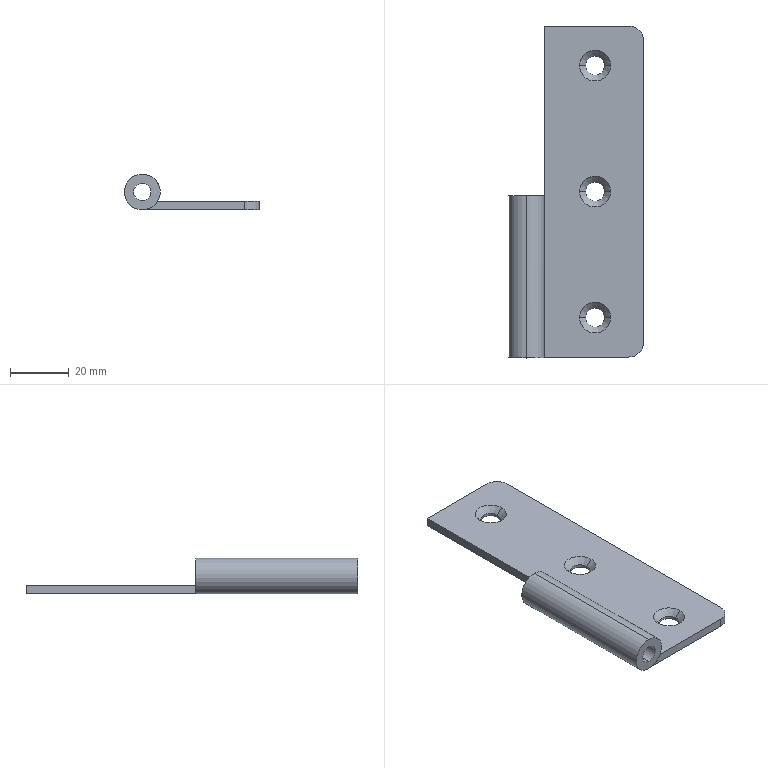Part | SolidWorks | features BaseBody 1 | 1 solid | 26 faces | box 46.1 x 113.3 x 12.2 mm | volume 16282 mm3 | cylinder 12 | plane 8 | cone 6 | commonest cylinder face diameters 6.5 x6 6 x2 10 x2 12.2 x2
STEP:
#1=CARTESIAN_POINT('',(20.25,43.,-6.1));
#2=VERTEX_POINT('',#1);
#3=CARTESIAN_POINT('',(26.75,43.,-6.1));
#4=VERTEX_POINT('',#3);
#5=CARTESIAN_POINT('',(23.5,43.,-6.1));
#6=DIRECTION('',(0.,0.,1.));
#7=DIRECTION('',(1.,0.,0.));
#8=AXIS2_PLACEMENT_3D('',#5,#6,#7);
#9=CIRCLE('',#8,3.25);
#10=EDGE_CURVE('',#2,#4,#9,.T.);
#11=ORIENTED_EDGE('',*,*,#10,.F.);
#12=CARTESIAN_POINT('',(20.25,43.,-5.15));
#13=VERTEX_POINT('',#12);
#14=CARTESIAN_POINT('',(20.25,43.,-3.1));
#15=DIRECTION('',(0.,0.,1.));
#16=VECTOR('',#15,1000.);
#17=LINE('',#14,#16);
#18=EDGE_CURVE('',#2,#13,#17,.T.);
#19=ORIENTED_EDGE('',*,*,#18,.T.);
#20=CARTESIAN_POINT('',(26.75,43.,-5.15));
#21=VERTEX_POINT('',#20);
#22=CARTESIAN_POINT('',(23.5,43.,-5.15));
#23=DIRECTION('',(0.,0.,1.));
#24=DIRECTION('',(1.,0.,0.));
#25=AXIS2_PLACEMENT_3D('',#22,#23,#24);
#26=CIRCLE('',#25,3.25);
#27=EDGE_CURVE('',#13,#21,#26,.T.);
#28=ORIENTED_EDGE('',*,*,#27,.T.);
#29=CARTESIAN_POINT('',(26.75,43.,-3.1));
#30=DIRECTION('',(0.,0.,1.));
#31=VECTOR('',#30,1000.);
#32=LINE('',#29,#31);
#33=EDGE_CURVE('',#4,#21,#32,.T.);
#34=ORIENTED_EDGE('',*,*,#33,.F.);
#35=EDGE_LOOP('',(#11,#19,#28,#34));
#36=FACE_OUTER_BOUND('',#35,.T.);
#37=CARTESIAN_POINT('',(23.5,43.,-3.1));
#38=DIRECTION('',(0.,0.,1.));
#39=DIRECTION('',(1.,0.,0.));
#40=AXIS2_PLACEMENT_3D('',#37,#38,#39);
#41=CYLINDRICAL_SURFACE('',#40,3.25);
#42=ADVANCED_FACE('',(#36),#41,.F.);
#43=CARTESIAN_POINT('',(20.25,0.,-6.1));
#44=VERTEX_POINT('',#43);
#45=CARTESIAN_POINT('',(26.75,0.,-6.1));
#46=VERTEX_POINT('',#45);
#47=CARTESIAN_POINT('',(23.5,0.,-6.1));
#48=DIRECTION('',(0.,0.,1.));
#49=DIRECTION('',(1.,0.,0.));
#50=AXIS2_PLACEMENT_3D('',#47,#48,#49);
#51=CIRCLE('',#50,3.25);
#52=EDGE_CURVE('',#44,#46,#51,.T.);
#53=ORIENTED_EDGE('',*,*,#52,.F.);
#54=CARTESIAN_POINT('',(20.25,0.,-5.15));
#55=VERTEX_POINT('',#54);
#56=CARTESIAN_POINT('',(20.25,0.,-3.1));
#57=DIRECTION('',(0.,0.,1.));
#58=VECTOR('',#57,1000.);
#59=LINE('',#56,#58);
#60=EDGE_CURVE('',#44,#55,#59,.T.);
#61=ORIENTED_EDGE('',*,*,#60,.T.);
#62=CARTESIAN_POINT('',(26.75,0.,-5.15));
#63=VERTEX_POINT('',#62);
#64=CARTESIAN_POINT('',(23.5,0.,-5.15));
#65=DIRECTION('',(0.,0.,1.));
#66=DIRECTION('',(1.,0.,0.));
#67=AXIS2_PLACEMENT_3D('',#64,#65,#66);
#68=CIRCLE('',#67,3.25);
#69=EDGE_CURVE('',#55,#63,#68,.T.);
#70=ORIENTED_EDGE('',*,*,#69,.T.);
#71=CARTESIAN_POINT('',(26.75,0.,-3.1));
#72=DIRECTION('',(0.,0.,1.));
#73=VECTOR('',#72,1000.);
#74=LINE('',#71,#73);
#75=EDGE_CURVE('',#46,#63,#74,.T.);
#76=ORIENTED_EDGE('',*,*,#75,.F.);
#77=EDGE_LOOP('',(#53,#61,#70,#76));
#78=FACE_OUTER_BOUND('',#77,.T.);
#79=CARTESIAN_POINT('',(23.5,0.,-3.1));
#80=DIRECTION('',(0.,0.,1.));
#81=DIRECTION('',(1.,0.,0.));
#82=AXIS2_PLACEMENT_3D('',#79,#80,#81);
#83=CYLINDRICAL_SURFACE('',#82,3.25);
#84=ADVANCED_FACE('',(#78),#83,.F.);
#85=CARTESIAN_POINT('',(20.25,-43.,-6.1));
#86=VERTEX_POINT('',#85);
#87=CARTESIAN_POINT('',(26.75,-43.,-6.1));
#88=VERTEX_POINT('',#87);
#89=CARTESIAN_POINT('',(23.5,-43.,-6.1));
#90=DIRECTION('',(0.,0.,1.));
#91=DIRECTION('',(1.,0.,0.));
#92=AXIS2_PLACEMENT_3D('',#89,#90,#91);
#93=CIRCLE('',#92,3.25);
#94=EDGE_CURVE('',#86,#88,#93,.T.);
#95=ORIENTED_EDGE('',*,*,#94,.F.);
#96=CARTESIAN_POINT('',(20.25,-43.,-5.15));
#97=VERTEX_POINT('',#96);
#98=CARTESIAN_POINT('',(20.25,-43.,-3.1));
#99=DIRECTION('',(0.,0.,1.));
#100=VECTOR('',#99,1000.);
#101=LINE('',#98,#100);
#102=EDGE_CURVE('',#86,#97,#101,.T.);
#103=ORIENTED_EDGE('',*,*,#102,.T.);
#104=CARTESIAN_POINT('',(26.75,-43.,-5.15));
#105=VERTEX_POINT('',#104);
#106=CARTESIAN_POINT('',(23.5,-43.,-5.15));
#107=DIRECTION('',(0.,0.,1.));
#108=DIRECTION('',(1.,0.,0.));
#109=AXIS2_PLACEMENT_3D('',#106,#107,#108);
#110=CIRCLE('',#109,3.25);
#111=EDGE_CURVE('',#97,#105,#110,.T.);
#112=ORIENTED_EDGE('',*,*,#111,.T.);
#113=CARTESIAN_POINT('',(26.75,-43.,-3.1));
#114=DIRECTION('',(0.,0.,1.));
#115=VECTOR('',#114,1000.);
#116=LINE('',#113,#115);
#117=EDGE_CURVE('',#88,#105,#116,.T.);
#118=ORIENTED_EDGE('',*,*,#117,.F.);
#119=EDGE_LOOP('',(#95,#103,#112,#118));
#120=FACE_OUTER_BOUND('',#119,.T.);
#121=CARTESIAN_POINT('',(23.5,-43.,-3.1));
#122=DIRECTION('',(0.,0.,1.));
#123=DIRECTION('',(1.,0.,0.));
#124=AXIS2_PLACEMENT_3D('',#121,#122,#123);
#125=CYLINDRICAL_SURFACE('',#124,3.25);
#126=ADVANCED_FACE('',(#120),#125,.F.);
#127=ORIENTED_EDGE('',*,*,#27,.F.);
#128=CARTESIAN_POINT('',(18.2,43.,-3.1));
#129=VERTEX_POINT('',#128);
#130=CARTESIAN_POINT('',(20.25,43.,-5.15));
#131=DIRECTION('',(-0.7071,0.,0.7071));
#132=VECTOR('',#131,1000.);
#133=LINE('',#130,#132);
#134=EDGE_CURVE('',#13,#129,#133,.T.);
#135=ORIENTED_EDGE('',*,*,#134,.T.);
#136=CARTESIAN_POINT('',(28.8,43.,-3.1));
#137=VERTEX_POINT('',#136);
#138=CARTESIAN_POINT('',(23.5,43.,-3.1));
#139=DIRECTION('',(0.,0.,1.));
#140=DIRECTION('',(1.,0.,0.));
#141=AXIS2_PLACEMENT_3D('',#138,#139,#140);
#142=CIRCLE('',#141,5.3);
#143=EDGE_CURVE('',#129,#137,#142,.T.);
#144=ORIENTED_EDGE('',*,*,#143,.T.);
#145=CARTESIAN_POINT('',(26.75,43.,-5.15));
#146=DIRECTION('',(0.7071,0.,0.7071));
#147=VECTOR('',#146,1000.);
#148=LINE('',#145,#147);
#149=EDGE_CURVE('',#21,#137,#148,.T.);
#150=ORIENTED_EDGE('',*,*,#149,.F.);
#151=EDGE_LOOP('',(#127,#135,#144,#150));
#152=FACE_OUTER_BOUND('',#151,.T.);
#153=CARTESIAN_POINT('',(23.5,43.,-5.15));
#154=DIRECTION('',(0.,0.,1.));
#155=DIRECTION('',(1.,0.,0.));
#156=AXIS2_PLACEMENT_3D('',#153,#154,#155);
#157=CONICAL_SURFACE('',#156,3.25,0.7854);
#158=ADVANCED_FACE('',(#152),#157,.F.);
#159=ORIENTED_EDGE('',*,*,#69,.F.);
#160=CARTESIAN_POINT('',(18.2,0.,-3.1));
#161=VERTEX_POINT('',#160);
#162=CARTESIAN_POINT('',(20.25,0.,-5.15));
#163=DIRECTION('',(-0.7071,0.,0.7071));
#164=VECTOR('',#163,1000.);
#165=LINE('',#162,#164);
#166=EDGE_CURVE('',#55,#161,#165,.T.);
#167=ORIENTED_EDGE('',*,*,#166,.T.);
#168=CARTESIAN_POINT('',(28.8,0.,-3.1));
#169=VERTEX_POINT('',#168);
#170=CARTESIAN_POINT('',(23.5,0.,-3.1));
#171=DIRECTION('',(0.,0.,1.));
#172=DIRECTION('',(1.,0.,0.));
#173=AXIS2_PLACEMENT_3D('',#170,#171,#172);
#174=CIRCLE('',#173,5.3);
#175=EDGE_CURVE('',#161,#169,#174,.T.);
#176=ORIENTED_EDGE('',*,*,#175,.T.);
#177=CARTESIAN_POINT('',(26.75,0.,-5.15));
#178=DIRECTION('',(0.7071,0.,0.7071));
#179=VECTOR('',#178,1000.);
#180=LINE('',#177,#179);
#181=EDGE_CURVE('',#63,#169,#180,.T.);
#182=ORIENTED_EDGE('',*,*,#181,.F.);
#183=EDGE_LOOP('',(#159,#167,#176,#182));
#184=FACE_OUTER_BOUND('',#183,.T.);
#185=CARTESIAN_POINT('',(23.5,0.,-5.15));
#186=DIRECTION('',(0.,0.,1.));
#187=DIRECTION('',(1.,0.,0.));
#188=AXIS2_PLACEMENT_3D('',#185,#186,#187);
#189=CONICAL_SURFACE('',#188,3.25,0.7854);
#190=ADVANCED_FACE('',(#184),#189,.F.);
#191=ORIENTED_EDGE('',*,*,#111,.F.);
#192=CARTESIAN_POINT('',(18.2,-43.,-3.1));
#193=VERTEX_POINT('',#192);
#194=CARTESIAN_POINT('',(20.25,-43.,-5.15));
#195=DIRECTION('',(-0.7071,0.,0.7071));
#196=VECTOR('',#195,1000.);
#197=LINE('',#194,#196);
#198=EDGE_CURVE('',#97,#193,#197,.T.);
#199=ORIENTED_EDGE('',*,*,#198,.T.);
#200=CARTESIAN_POINT('',(28.8,-43.,-3.1));
#201=VERTEX_POINT('',#200);
#202=CARTESIAN_POINT('',(23.5,-43.,-3.1));
#203=DIRECTION('',(0.,0.,1.));
#204=DIRECTION('',(1.,0.,0.));
#205=AXIS2_PLACEMENT_3D('',#202,#203,#204);
#206=CIRCLE('',#205,5.3);
#207=EDGE_CURVE('',#193,#201,#206,.T.);
#208=ORIENTED_EDGE('',*,*,#207,.T.);
#209=CARTESIAN_POINT('',(26.75,-43.,-5.15));
#210=DIRECTION('',(0.7071,0.,0.7071));
#211=VECTOR('',#210,1000.);
#212=LINE('',#209,#211);
#213=EDGE_CURVE('',#105,#201,#212,.T.);
#214=ORIENTED_EDGE('',*,*,#213,.F.);
#215=EDGE_LOOP('',(#191,#199,#208,#214));
#216=FACE_OUTER_BOUND('',#215,.T.);
#217=CARTESIAN_POINT('',(23.5,-43.,-5.15));
#218=DIRECTION('',(0.,0.,1.));
#219=DIRECTION('',(1.,0.,0.));
#220=AXIS2_PLACEMENT_3D('',#217,#218,#219);
#221=CONICAL_SURFACE('',#220,3.25,0.7854);
#222=ADVANCED_FACE('',(#216),#221,.F.);
#223=CARTESIAN_POINT('',(0.,-1.5,3.));
#224=VERTEX_POINT('',#223);
#225=CARTESIAN_POINT('',(0.,-1.5,-3.));
#226=VERTEX_POINT('',#225);
#227=CARTESIAN_POINT('',(0.,-1.5,0.));
#228=DIRECTION('',(0.,-1.,0.));
#229=DIRECTION('',(0.,0.,1.));
#230=AXIS2_PLACEMENT_3D('',#227,#228,#229);
#231=CIRCLE('',#230,3.);
#232=EDGE_CURVE('',#224,#226,#231,.T.);
#233=ORIENTED_EDGE('',*,*,#232,.F.);
#234=CARTESIAN_POINT('',(0.,-56.8,3.));
#235=VERTEX_POINT('',#234);
#236=CARTESIAN_POINT('',(0.,-56.8,3.));
#237=DIRECTION('',(0.,-1.,0.));
#238=VECTOR('',#237,1000.);
#239=LINE('',#236,#238);
#240=EDGE_CURVE('',#224,#235,#239,.T.);
#241=ORIENTED_EDGE('',*,*,#240,.T.);
#242=CARTESIAN_POINT('',(0.,-56.8,-3.));
#243=VERTEX_POINT('',#242);
#244=CARTESIAN_POINT('',(0.,-56.8,0.));
#245=DIRECTION('',(0.,-1.,0.));
#246=DIRECTION('',(0.,0.,-1.));
#247=AXIS2_PLACEMENT_3D('',#244,#245,#246);
#248=CIRCLE('',#247,3.);
#249=EDGE_CURVE('',#235,#243,#248,.T.);
#250=ORIENTED_EDGE('',*,*,#249,.T.);
#251=CARTESIAN_POINT('',(0.,-56.8,-3.));
#252=DIRECTION('',(0.,-1.,0.));
#253=VECTOR('',#252,1000.);
#254=LINE('',#251,#253);
#255=EDGE_CURVE('',#226,#243,#254,.T.);
#256=ORIENTED_EDGE('',*,*,#255,.F.);
#257=EDGE_LOOP('',(#233,#241,#250,#256));
#258=FACE_OUTER_BOUND('',#257,.T.);
#259=CARTESIAN_POINT('',(0.,-56.8,0.));
#260=DIRECTION('',(0.,-1.,0.));
#261=DIRECTION('',(0.,0.,-1.));
#262=AXIS2_PLACEMENT_3D('',#259,#260,#261);
#263=CYLINDRICAL_SURFACE('',#262,3.);
#264=ADVANCED_FACE('',(#258),#263,.F.);
#265=CARTESIAN_POINT('',(0.,-1.5,6.1));
#266=VERTEX_POINT('',#265);
#267=CARTESIAN_POINT('',(5.254,-1.5,-3.1));
#268=VERTEX_POINT('',#267);
#269=CARTESIAN_POINT('',(0.,-1.5,0.));
#270=DIRECTION('',(0.,1.,0.));
#271=DIRECTION('',(0.,0.,-1.));
#272=AXIS2_PLACEMENT_3D('',#269,#270,#271);
#273=CIRCLE('',#272,6.1);
#274=EDGE_CURVE('',#266,#268,#273,.T.);
#275=ORIENTED_EDGE('',*,*,#274,.F.);
#276=CARTESIAN_POINT('',(0.,-56.8,6.1));
#277=VERTEX_POINT('',#276);
#278=CARTESIAN_POINT('',(0.,-56.8,6.1));
#279=DIRECTION('',(0.,-1.,0.));
#280=VECTOR('',#279,1000.);
#281=LINE('',#278,#280);
#282=EDGE_CURVE('',#266,#277,#281,.T.);
#283=ORIENTED_EDGE('',*,*,#282,.T.);
#284=CARTESIAN_POINT('',(0.,-56.8,-6.1));
#285=VERTEX_POINT('',#284);
#286=CARTESIAN_POINT('',(0.,-56.8,0.));
#287=DIRECTION('',(0.,-1.,0.));
#288=DIRECTION('',(0.,0.,-1.));
#289=AXIS2_PLACEMENT_3D('',#286,#287,#288);
#290=CIRCLE('',#289,6.1);
#291=EDGE_CURVE('',#285,#277,#290,.T.);
#292=ORIENTED_EDGE('',*,*,#291,.F.);
#293=CARTESIAN_POINT('',(0.,-56.5,-6.1));
#294=VERTEX_POINT('',#293);
#295=CARTESIAN_POINT('',(0.,-56.8,-6.1));
#296=DIRECTION('',(0.,-1.,0.));
#297=VECTOR('',#296,1000.);
#298=LINE('',#295,#297);
#299=EDGE_CURVE('',#294,#285,#298,.T.);
#300=ORIENTED_EDGE('',*,*,#299,.F.);
#301=CARTESIAN_POINT('',(5.254,-56.5,-3.1));
#302=VERTEX_POINT('',#301);
#303=CARTESIAN_POINT('',(0.,-56.5,0.));
#304=DIRECTION('',(0.,1.,0.));
#305=DIRECTION('',(0.8612,0.,-0.5082));
#306=AXIS2_PLACEMENT_3D('',#303,#304,#305);
#307=CIRCLE('',#306,6.1);
#308=EDGE_CURVE('',#302,#294,#307,.T.);
#309=ORIENTED_EDGE('',*,*,#308,.F.);
#310=CARTESIAN_POINT('',(5.254,-56.5,-3.1));
#311=DIRECTION('',(0.,1.,0.));
#312=VECTOR('',#311,1000.);
#313=LINE('',#310,#312);
#314=EDGE_CURVE('',#302,#268,#313,.T.);
#315=ORIENTED_EDGE('',*,*,#314,.T.);
#316=EDGE_LOOP('',(#275,#283,#292,#300,#309,#315));
#317=FACE_OUTER_BOUND('',#316,.T.);
#318=CARTESIAN_POINT('',(0.,-56.8,0.));
#319=DIRECTION('',(0.,-1.,0.));
#320=DIRECTION('',(0.,0.,-1.));
#321=AXIS2_PLACEMENT_3D('',#318,#319,#320);
#322=CYLINDRICAL_SURFACE('',#321,6.1);
#323=ADVANCED_FACE('',(#317),#322,.T.);
#324=ORIENTED_EDGE('',*,*,#282,.F.);
#325=CARTESIAN_POINT('',(0.,-1.5,-6.1));
#326=VERTEX_POINT('',#325);
#327=CARTESIAN_POINT('',(0.,-1.5,0.));
#328=DIRECTION('',(0.,1.,0.));
#329=DIRECTION('',(0.,0.,-1.));
#330=AXIS2_PLACEMENT_3D('',#327,#328,#329);
#331=CIRCLE('',#330,6.1);
#332=EDGE_CURVE('',#326,#266,#331,.T.);
#333=ORIENTED_EDGE('',*,*,#332,.F.);
#334=CARTESIAN_POINT('',(0.,-1.5,-6.1));
#335=DIRECTION('',(0.,-1.,0.));
#336=VECTOR('',#335,1000.);
#337=LINE('',#334,#336);
#338=EDGE_CURVE('',#326,#294,#337,.T.);
#339=ORIENTED_EDGE('',*,*,#338,.T.);
#340=ORIENTED_EDGE('',*,*,#299,.T.);
#341=CARTESIAN_POINT('',(0.,-56.8,0.));
#342=DIRECTION('',(0.,-1.,0.));
#343=DIRECTION('',(0.,0.,-1.));
#344=AXIS2_PLACEMENT_3D('',#341,#342,#343);
#345=CIRCLE('',#344,6.1);
#346=EDGE_CURVE('',#277,#285,#345,.T.);
#347=ORIENTED_EDGE('',*,*,#346,.F.);
#348=EDGE_LOOP('',(#324,#333,#339,#340,#347));
#349=FACE_OUTER_BOUND('',#348,.T.);
#350=CARTESIAN_POINT('',(0.,-56.8,0.));
#351=DIRECTION('',(0.,-1.,0.));
#352=DIRECTION('',(0.,0.,-1.));
#353=AXIS2_PLACEMENT_3D('',#350,#351,#352);
#354=CYLINDRICAL_SURFACE('',#353,6.1);
#355=ADVANCED_FACE('',(#349),#354,.T.);
#356=CARTESIAN_POINT('',(0.,-56.8,0.));
#357=DIRECTION('',(0.,-1.,0.));
#358=DIRECTION('',(0.,0.,-1.));
#359=AXIS2_PLACEMENT_3D('',#356,#357,#358);
#360=CIRCLE('',#359,3.);
#361=EDGE_CURVE('',#243,#235,#360,.T.);
#362=ORIENTED_EDGE('',*,*,#361,.F.);
#363=ORIENTED_EDGE('',*,*,#249,.F.);
#364=EDGE_LOOP('',(#362,#363));
#365=FACE_BOUND('',#364,.T.);
#366=ORIENTED_EDGE('',*,*,#291,.T.);
#367=ORIENTED_EDGE('',*,*,#346,.T.);
#368=EDGE_LOOP('',(#366,#367));
#369=FACE_OUTER_BOUND('',#368,.T.);
#370=CARTESIAN_POINT('',(6.1,-56.8,0.));
#371=DIRECTION('',(0.,1.,0.));
#372=DIRECTION('',(0.,0.,1.));
#373=AXIS2_PLACEMENT_3D('',#370,#371,#372);
#374=PLANE('',#373);
#375=ADVANCED_FACE('',(#365,#369),#374,.F.);
#376=CARTESIAN_POINT('',(23.5,-43.,-3.1));
#377=DIRECTION('',(0.,0.,1.));
#378=DIRECTION('',(1.,0.,0.));
#379=AXIS2_PLACEMENT_3D('',#376,#377,#378);
#380=CIRCLE('',#379,5.3);
#381=EDGE_CURVE('',#201,#193,#380,.T.);
#382=ORIENTED_EDGE('',*,*,#381,.F.);
#383=ORIENTED_EDGE('',*,*,#207,.F.);
#384=EDGE_LOOP('',(#382,#383));
#385=FACE_BOUND('',#384,.T.);
#386=CARTESIAN_POINT('',(23.5,0.,-3.1));
#387=DIRECTION('',(0.,0.,1.));
#388=DIRECTION('',(1.,0.,0.));
#389=AXIS2_PLACEMENT_3D('',#386,#387,#388);
#390=CIRCLE('',#389,5.3);
#391=EDGE_CURVE('',#169,#161,#390,.T.);
#392=ORIENTED_EDGE('',*,*,#391,.F.);
#393=ORIENTED_EDGE('',*,*,#175,.F.);
#394=EDGE_LOOP('',(#392,#393));
#395=FACE_BOUND('',#394,.T.);
#396=CARTESIAN_POINT('',(23.5,43.,-3.1));
#397=DIRECTION('',(0.,0.,1.));
#398=DIRECTION('',(1.,0.,0.));
#399=AXIS2_PLACEMENT_3D('',#396,#397,#398);
#400=CIRCLE('',#399,5.3);
#401=EDGE_CURVE('',#137,#129,#400,.T.);
#402=ORIENTED_EDGE('',*,*,#401,.F.);
#403=ORIENTED_EDGE('',*,*,#143,.F.);
#404=EDGE_LOOP('',(#402,#403));
#405=FACE_BOUND('',#404,.T.);
#406=CARTESIAN_POINT('',(6.2,56.5,-3.1));
#407=VERTEX_POINT('',#406);
#408=CARTESIAN_POINT('',(6.2,-1.5,-3.1));
#409=VERTEX_POINT('',#408);
#410=CARTESIAN_POINT('',(6.2,56.5,-3.1));
#411=DIRECTION('',(0.,-1.,0.));
#412=VECTOR('',#411,1000.);
#413=LINE('',#410,#412);
#414=EDGE_CURVE('',#407,#409,#413,.T.);
#415=ORIENTED_EDGE('',*,*,#414,.T.);
#416=CARTESIAN_POINT('',(6.2,-1.5,-3.1));
#417=DIRECTION('',(-1.,0.,0.));
#418=VECTOR('',#417,1000.);
#419=LINE('',#416,#418);
#420=EDGE_CURVE('',#409,#268,#419,.T.);
#421=ORIENTED_EDGE('',*,*,#420,.T.);
#422=ORIENTED_EDGE('',*,*,#314,.F.);
#423=CARTESIAN_POINT('',(35.,-56.5,-3.1));
#424=VERTEX_POINT('',#423);
#425=CARTESIAN_POINT('',(5.254,-56.5,-3.1));
#426=DIRECTION('',(1.,0.,0.));
#427=VECTOR('',#426,1000.);
#428=LINE('',#425,#427);
#429=EDGE_CURVE('',#302,#424,#428,.T.);
#430=ORIENTED_EDGE('',*,*,#429,.T.);
#431=CARTESIAN_POINT('',(40.,-51.5,-3.1));
#432=VERTEX_POINT('',#431);
#433=CARTESIAN_POINT('',(35.,-51.5,-3.1));
#434=DIRECTION('',(0.,0.,1.));
#435=DIRECTION('',(0.,-1.,0.));
#436=AXIS2_PLACEMENT_3D('',#433,#434,#435);
#437=CIRCLE('',#436,5.);
#438=EDGE_CURVE('',#424,#432,#437,.T.);
#439=ORIENTED_EDGE('',*,*,#438,.T.);
#440=CARTESIAN_POINT('',(40.,51.5,-3.1));
#441=VERTEX_POINT('',#440);
#442=CARTESIAN_POINT('',(40.,-51.5,-3.1));
#443=DIRECTION('',(0.,1.,0.));
#444=VECTOR('',#443,1000.);
#445=LINE('',#442,#444);
#446=EDGE_CURVE('',#432,#441,#445,.T.);
#447=ORIENTED_EDGE('',*,*,#446,.T.);
#448=CARTESIAN_POINT('',(35.,56.5,-3.1));
#449=VERTEX_POINT('',#448);
#450=CARTESIAN_POINT('',(35.,51.5,-3.1));
#451=DIRECTION('',(0.,0.,1.));
#452=DIRECTION('',(1.,0.,0.));
#453=AXIS2_PLACEMENT_3D('',#450,#451,#452);
#454=CIRCLE('',#453,5.);
#455=EDGE_CURVE('',#441,#449,#454,.T.);
#456=ORIENTED_EDGE('',*,*,#455,.T.);
#457=CARTESIAN_POINT('',(35.,56.5,-3.1));
#458=DIRECTION('',(-1.,0.,0.));
#459=VECTOR('',#458,1000.);
#460=LINE('',#457,#459);
#461=EDGE_CURVE('',#449,#407,#460,.T.);
#462=ORIENTED_EDGE('',*,*,#461,.T.);
#463=EDGE_LOOP('',(#415,#421,#422,#430,#439,#447,#456,#462));
#464=FACE_OUTER_BOUND('',#463,.T.);
#465=CARTESIAN_POINT('',(35.,-51.5,-3.1));
#466=DIRECTION('',(0.,0.,1.));
#467=DIRECTION('',(1.,0.,0.));
#468=AXIS2_PLACEMENT_3D('',#465,#466,#467);
#469=PLANE('',#468);
#470=ADVANCED_FACE('',(#385,#395,#405,#464),#469,.T.);
#471=CARTESIAN_POINT('',(0.,-1.5,0.));
#472=DIRECTION('',(0.,-1.,0.));
#473=DIRECTION('',(0.,0.,1.));
#474=AXIS2_PLACEMENT_3D('',#471,#472,#473);
#475=CIRCLE('',#474,3.);
#476=EDGE_CURVE('',#226,#224,#475,.T.);
#477=ORIENTED_EDGE('',*,*,#476,.T.);
#478=ORIENTED_EDGE('',*,*,#232,.T.);
#479=EDGE_LOOP('',(#477,#478));
#480=FACE_BOUND('',#479,.T.);
#481=CARTESIAN_POINT('',(6.2,-1.5,-6.1));
#482=VERTEX_POINT('',#481);
#483=CARTESIAN_POINT('',(6.2,-1.5,-3.1));
#484=DIRECTION('',(0.,0.,-1.));
#485=VECTOR('',#484,1000.);
#486=LINE('',#483,#485);
#487=EDGE_CURVE('',#409,#482,#486,.T.);
#488=ORIENTED_EDGE('',*,*,#487,.T.);
#489=CARTESIAN_POINT('',(6.2,-1.5,-6.1));
#490=DIRECTION('',(-1.,0.,0.));
#491=VECTOR('',#490,1000.);
#492=LINE('',#489,#491);
#493=EDGE_CURVE('',#482,#326,#492,.T.);
#494=ORIENTED_EDGE('',*,*,#493,.T.);
#495=ORIENTED_EDGE('',*,*,#332,.T.);
#496=ORIENTED_EDGE('',*,*,#274,.T.);
#497=ORIENTED_EDGE('',*,*,#420,.F.);
#498=EDGE_LOOP('',(#488,#494,#495,#496,#497));
#499=FACE_OUTER_BOUND('',#498,.T.);
#500=CARTESIAN_POINT('',(-6.35,-1.5,12.2));
#501=DIRECTION('',(0.,1.,0.));
#502=DIRECTION('',(0.,0.,1.));
#503=AXIS2_PLACEMENT_3D('',#500,#501,#502);
#504=PLANE('',#503);
#505=ADVANCED_FACE('',(#480,#499),#504,.T.);
#506=CARTESIAN_POINT('',(23.5,-43.,-6.1));
#507=DIRECTION('',(0.,0.,1.));
#508=DIRECTION('',(1.,0.,0.));
#509=AXIS2_PLACEMENT_3D('',#506,#507,#508);
#510=CIRCLE('',#509,3.25);
#511=EDGE_CURVE('',#88,#86,#510,.T.);
#512=ORIENTED_EDGE('',*,*,#511,.T.);
#513=ORIENTED_EDGE('',*,*,#94,.T.);
#514=EDGE_LOOP('',(#512,#513));
#515=FACE_BOUND('',#514,.T.);
#516=CARTESIAN_POINT('',(23.5,0.,-6.1));
#517=DIRECTION('',(0.,0.,1.));
#518=DIRECTION('',(1.,0.,0.));
#519=AXIS2_PLACEMENT_3D('',#516,#517,#518);
#520=CIRCLE('',#519,3.25);
#521=EDGE_CURVE('',#46,#44,#520,.T.);
#522=ORIENTED_EDGE('',*,*,#521,.T.);
#523=ORIENTED_EDGE('',*,*,#52,.T.);
#524=EDGE_LOOP('',(#522,#523));
#525=FACE_BOUND('',#524,.T.);
#526=CARTESIAN_POINT('',(23.5,43.,-6.1));
#527=DIRECTION('',(0.,0.,1.));
#528=DIRECTION('',(1.,0.,0.));
#529=AXIS2_PLACEMENT_3D('',#526,#527,#528);
#530=CIRCLE('',#529,3.25);
#531=EDGE_CURVE('',#4,#2,#530,.T.);
#532=ORIENTED_EDGE('',*,*,#531,.T.);
#533=ORIENTED_EDGE('',*,*,#10,.T.);
#534=EDGE_LOOP('',(#532,#533));
#535=FACE_BOUND('',#534,.T.);
#536=ORIENTED_EDGE('',*,*,#493,.F.);
#537=CARTESIAN_POINT('',(6.2,56.5,-6.1));
#538=VERTEX_POINT('',#537);
#539=CARTESIAN_POINT('',(6.2,56.5,-6.1));
#540=DIRECTION('',(0.,-1.,0.));
#541=VECTOR('',#540,1000.);
#542=LINE('',#539,#541);
#543=EDGE_CURVE('',#538,#482,#542,.T.);
#544=ORIENTED_EDGE('',*,*,#543,.F.);
#545=CARTESIAN_POINT('',(35.,56.5,-6.1));
#546=VERTEX_POINT('',#545);
#547=CARTESIAN_POINT('',(35.,56.5,-6.1));
#548=DIRECTION('',(-1.,0.,0.));
#549=VECTOR('',#548,1000.);
#550=LINE('',#547,#549);
#551=EDGE_CURVE('',#546,#538,#550,.T.);
#552=ORIENTED_EDGE('',*,*,#551,.F.);
#553=CARTESIAN_POINT('',(40.,51.5,-6.1));
#554=VERTEX_POINT('',#553);
#555=CARTESIAN_POINT('',(35.,51.5,-6.1));
#556=DIRECTION('',(0.,0.,1.));
#557=DIRECTION('',(1.,0.,0.));
#558=AXIS2_PLACEMENT_3D('',#555,#556,#557);
#559=CIRCLE('',#558,5.);
#560=EDGE_CURVE('',#554,#546,#559,.T.);
#561=ORIENTED_EDGE('',*,*,#560,.F.);
#562=CARTESIAN_POINT('',(40.,-51.5,-6.1));
#563=VERTEX_POINT('',#562);
#564=CARTESIAN_POINT('',(40.,-51.5,-6.1));
#565=DIRECTION('',(0.,1.,0.));
#566=VECTOR('',#565,1000.);
#567=LINE('',#564,#566);
#568=EDGE_CURVE('',#563,#554,#567,.T.);
#569=ORIENTED_EDGE('',*,*,#568,.F.);
#570=CARTESIAN_POINT('',(35.,-56.5,-6.1));
#571=VERTEX_POINT('',#570);
#572=CARTESIAN_POINT('',(35.,-51.5,-6.1));
#573=DIRECTION('',(0.,0.,1.));
#574=DIRECTION('',(0.,-1.,0.));
#575=AXIS2_PLACEMENT_3D('',#572,#573,#574);
#576=CIRCLE('',#575,5.);
#577=EDGE_CURVE('',#571,#563,#576,.T.);
#578=ORIENTED_EDGE('',*,*,#577,.F.);
#579=CARTESIAN_POINT('',(0.,-56.5,-6.1));
#580=DIRECTION('',(1.,0.,0.));
#581=VECTOR('',#580,1000.);
#582=LINE('',#579,#581);
#583=EDGE_CURVE('',#294,#571,#582,.T.);
#584=ORIENTED_EDGE('',*,*,#583,.F.);
#585=ORIENTED_EDGE('',*,*,#338,.F.);
#586=EDGE_LOOP('',(#536,#544,#552,#561,#569,#578,#584,#585));
#587=FACE_OUTER_BOUND('',#586,.T.);
#588=CARTESIAN_POINT('',(35.,-51.5,-6.1));
#589=DIRECTION('',(0.,0.,1.));
#590=DIRECTION('',(1.,0.,0.));
#591=AXIS2_PLACEMENT_3D('',#588,#589,#590);
#592=PLANE('',#591);
#593=ADVANCED_FACE('',(#515,#525,#535,#587),#592,.F.);
#594=ORIENTED_EDGE('',*,*,#429,.F.);
#595=ORIENTED_EDGE('',*,*,#308,.T.);
#596=ORIENTED_EDGE('',*,*,#583,.T.);
#597=CARTESIAN_POINT('',(35.,-56.5,-3.1));
#598=DIRECTION('',(0.,0.,-1.));
#599=VECTOR('',#598,1000.);
#600=LINE('',#597,#599);
#601=EDGE_CURVE('',#424,#571,#600,.T.);
#602=ORIENTED_EDGE('',*,*,#601,.F.);
#603=EDGE_LOOP('',(#594,#595,#596,#602));
#604=FACE_OUTER_BOUND('',#603,.T.);
#605=CARTESIAN_POINT('',(0.,-56.5,-3.1));
#606=DIRECTION('',(0.,1.,0.));
#607=DIRECTION('',(0.,0.,1.));
#608=AXIS2_PLACEMENT_3D('',#605,#606,#607);
#609=PLANE('',#608);
#610=ADVANCED_FACE('',(#604),#609,.F.);
#611=ORIENTED_EDGE('',*,*,#240,.F.);
#612=ORIENTED_EDGE('',*,*,#476,.F.);
#613=ORIENTED_EDGE('',*,*,#255,.T.);
#614=ORIENTED_EDGE('',*,*,#361,.T.);
#615=EDGE_LOOP('',(#611,#612,#613,#614));
#616=FACE_OUTER_BOUND('',#615,.T.);
#617=CARTESIAN_POINT('',(0.,-56.8,0.));
#618=DIRECTION('',(0.,-1.,0.));
#619=DIRECTION('',(0.,0.,-1.));
#620=AXIS2_PLACEMENT_3D('',#617,#618,#619);
#621=CYLINDRICAL_SURFACE('',#620,3.);
#622=ADVANCED_FACE('',(#616),#621,.F.);
#623=ORIENTED_EDGE('',*,*,#198,.F.);
#624=CARTESIAN_POINT('',(23.5,-43.,-5.15));
#625=DIRECTION('',(0.,0.,1.));
#626=DIRECTION('',(1.,0.,0.));
#627=AXIS2_PLACEMENT_3D('',#624,#625,#626);
#628=CIRCLE('',#627,3.25);
#629=EDGE_CURVE('',#105,#97,#628,.T.);
#630=ORIENTED_EDGE('',*,*,#629,.F.);
#631=ORIENTED_EDGE('',*,*,#213,.T.);
#632=ORIENTED_EDGE('',*,*,#381,.T.);
#633=EDGE_LOOP('',(#623,#630,#631,#632));
#634=FACE_OUTER_BOUND('',#633,.T.);
#635=CARTESIAN_POINT('',(23.5,-43.,-5.15));
#636=DIRECTION('',(0.,0.,1.));
#637=DIRECTION('',(1.,0.,0.));
#638=AXIS2_PLACEMENT_3D('',#635,#636,#637);
#639=CONICAL_SURFACE('',#638,3.25,0.7854);
#640=ADVANCED_FACE('',(#634),#639,.F.);
#641=ORIENTED_EDGE('',*,*,#166,.F.);
#642=CARTESIAN_POINT('',(23.5,0.,-5.15));
#643=DIRECTION('',(0.,0.,1.));
#644=DIRECTION('',(1.,0.,0.));
#645=AXIS2_PLACEMENT_3D('',#642,#643,#644);
#646=CIRCLE('',#645,3.25);
#647=EDGE_CURVE('',#63,#55,#646,.T.);
#648=ORIENTED_EDGE('',*,*,#647,.F.);
#649=ORIENTED_EDGE('',*,*,#181,.T.);
#650=ORIENTED_EDGE('',*,*,#391,.T.);
#651=EDGE_LOOP('',(#641,#648,#649,#650));
#652=FACE_OUTER_BOUND('',#651,.T.);
#653=CARTESIAN_POINT('',(23.5,0.,-5.15));
#654=DIRECTION('',(0.,0.,1.));
#655=DIRECTION('',(1.,0.,0.));
#656=AXIS2_PLACEMENT_3D('',#653,#654,#655);
#657=CONICAL_SURFACE('',#656,3.25,0.7854);
#658=ADVANCED_FACE('',(#652),#657,.F.);
#659=ORIENTED_EDGE('',*,*,#134,.F.);
#660=CARTESIAN_POINT('',(23.5,43.,-5.15));
#661=DIRECTION('',(0.,0.,1.));
#662=DIRECTION('',(1.,0.,0.));
#663=AXIS2_PLACEMENT_3D('',#660,#661,#662);
#664=CIRCLE('',#663,3.25);
#665=EDGE_CURVE('',#21,#13,#664,.T.);
#666=ORIENTED_EDGE('',*,*,#665,.F.);
#667=ORIENTED_EDGE('',*,*,#149,.T.);
#668=ORIENTED_EDGE('',*,*,#401,.T.);
#669=EDGE_LOOP('',(#659,#666,#667,#668));
#670=FACE_OUTER_BOUND('',#669,.T.);
#671=CARTESIAN_POINT('',(23.5,43.,-5.15));
#672=DIRECTION('',(0.,0.,1.));
#673=DIRECTION('',(1.,0.,0.));
#674=AXIS2_PLACEMENT_3D('',#671,#672,#673);
#675=CONICAL_SURFACE('',#674,3.25,0.7854);
#676=ADVANCED_FACE('',(#670),#675,.F.);
#677=CARTESIAN_POINT('',(6.2,56.5,-3.1));
#678=DIRECTION('',(0.,0.,-1.));
#679=VECTOR('',#678,1000.);
#680=LINE('',#677,#679);
#681=EDGE_CURVE('',#407,#538,#680,.T.);
#682=ORIENTED_EDGE('',*,*,#681,.T.);
#683=ORIENTED_EDGE('',*,*,#543,.T.);
#684=ORIENTED_EDGE('',*,*,#487,.F.);
#685=ORIENTED_EDGE('',*,*,#414,.F.);
#686=EDGE_LOOP('',(#682,#683,#684,#685));
#687=FACE_OUTER_BOUND('',#686,.T.);
#688=CARTESIAN_POINT('',(6.2,-1.5,12.2));
#689=DIRECTION('',(-1.,0.,0.));
#690=DIRECTION('',(0.,0.,1.));
#691=AXIS2_PLACEMENT_3D('',#688,#689,#690);
#692=PLANE('',#691);
#693=ADVANCED_FACE('',(#687),#692,.T.);
#694=ORIENTED_EDGE('',*,*,#577,.T.);
#695=CARTESIAN_POINT('',(40.,-51.5,-3.1));
#696=DIRECTION('',(0.,0.,-1.));
#697=VECTOR('',#696,1000.);
#698=LINE('',#695,#697);
#699=EDGE_CURVE('',#432,#563,#698,.T.);
#700=ORIENTED_EDGE('',*,*,#699,.F.);
#701=ORIENTED_EDGE('',*,*,#438,.F.);
#702=ORIENTED_EDGE('',*,*,#601,.T.);
#703=EDGE_LOOP('',(#694,#700,#701,#702));
#704=FACE_OUTER_BOUND('',#703,.T.);
#705=CARTESIAN_POINT('',(35.,-51.5,-3.1));
#706=DIRECTION('',(0.,0.,-1.));
#707=DIRECTION('',(-1.,0.,0.));
#708=AXIS2_PLACEMENT_3D('',#705,#706,#707);
#709=CYLINDRICAL_SURFACE('',#708,5.);
#710=ADVANCED_FACE('',(#704),#709,.T.);
#711=ORIENTED_EDGE('',*,*,#568,.T.);
#712=CARTESIAN_POINT('',(40.,51.5,-3.1));
#713=DIRECTION('',(0.,0.,-1.));
#714=VECTOR('',#713,1000.);
#715=LINE('',#712,#714);
#716=EDGE_CURVE('',#441,#554,#715,.T.);
#717=ORIENTED_EDGE('',*,*,#716,.F.);
#718=ORIENTED_EDGE('',*,*,#446,.F.);
#719=ORIENTED_EDGE('',*,*,#699,.T.);
#720=EDGE_LOOP('',(#711,#717,#718,#719));
#721=FACE_OUTER_BOUND('',#720,.T.);
#722=CARTESIAN_POINT('',(40.,-51.5,-3.1));
#723=DIRECTION('',(-1.,0.,0.));
#724=DIRECTION('',(0.,0.,1.));
#725=AXIS2_PLACEMENT_3D('',#722,#723,#724);
#726=PLANE('',#725);
#727=ADVANCED_FACE('',(#721),#726,.F.);
#728=ORIENTED_EDGE('',*,*,#560,.T.);
#729=CARTESIAN_POINT('',(35.,56.5,-3.1));
#730=DIRECTION('',(0.,0.,-1.));
#731=VECTOR('',#730,1000.);
#732=LINE('',#729,#731);
#733=EDGE_CURVE('',#449,#546,#732,.T.);
#734=ORIENTED_EDGE('',*,*,#733,.F.);
#735=ORIENTED_EDGE('',*,*,#455,.F.);
#736=ORIENTED_EDGE('',*,*,#716,.T.);
#737=EDGE_LOOP('',(#728,#734,#735,#736));
#738=FACE_OUTER_BOUND('',#737,.T.);
#739=CARTESIAN_POINT('',(35.,51.5,-3.1));
#740=DIRECTION('',(0.,0.,-1.));
#741=DIRECTION('',(-1.,0.,0.));
#742=AXIS2_PLACEMENT_3D('',#739,#740,#741);
#743=CYLINDRICAL_SURFACE('',#742,5.);
#744=ADVANCED_FACE('',(#738),#743,.T.);
#745=ORIENTED_EDGE('',*,*,#681,.F.);
#746=ORIENTED_EDGE('',*,*,#461,.F.);
#747=ORIENTED_EDGE('',*,*,#733,.T.);
#748=ORIENTED_EDGE('',*,*,#551,.T.);
#749=EDGE_LOOP('',(#745,#746,#747,#748));
#750=FACE_OUTER_BOUND('',#749,.T.);
#751=CARTESIAN_POINT('',(35.,56.5,-3.1));
#752=DIRECTION('',(0.,-1.,0.));
#753=DIRECTION('',(0.,0.,-1.));
#754=AXIS2_PLACEMENT_3D('',#751,#752,#753);
#755=PLANE('',#754);
#756=ADVANCED_FACE('',(#750),#755,.F.);
#757=ORIENTED_EDGE('',*,*,#102,.F.);
#758=ORIENTED_EDGE('',*,*,#511,.F.);
#759=ORIENTED_EDGE('',*,*,#117,.T.);
#760=ORIENTED_EDGE('',*,*,#629,.T.);
#761=EDGE_LOOP('',(#757,#758,#759,#760));
#762=FACE_OUTER_BOUND('',#761,.T.);
#763=CARTESIAN_POINT('',(23.5,-43.,-3.1));
#764=DIRECTION('',(0.,0.,1.));
#765=DIRECTION('',(1.,0.,0.));
#766=AXIS2_PLACEMENT_3D('',#763,#764,#765);
#767=CYLINDRICAL_SURFACE('',#766,3.25);
#768=ADVANCED_FACE('',(#762),#767,.F.);
#769=ORIENTED_EDGE('',*,*,#60,.F.);
#770=ORIENTED_EDGE('',*,*,#521,.F.);
#771=ORIENTED_EDGE('',*,*,#75,.T.);
#772=ORIENTED_EDGE('',*,*,#647,.T.);
#773=EDGE_LOOP('',(#769,#770,#771,#772));
#774=FACE_OUTER_BOUND('',#773,.T.);
#775=CARTESIAN_POINT('',(23.5,0.,-3.1));
#776=DIRECTION('',(0.,0.,1.));
#777=DIRECTION('',(1.,0.,0.));
#778=AXIS2_PLACEMENT_3D('',#775,#776,#777);
#779=CYLINDRICAL_SURFACE('',#778,3.25);
#780=ADVANCED_FACE('',(#774),#779,.F.);
#781=ORIENTED_EDGE('',*,*,#18,.F.);
#782=ORIENTED_EDGE('',*,*,#531,.F.);
#783=ORIENTED_EDGE('',*,*,#33,.T.);
#784=ORIENTED_EDGE('',*,*,#665,.T.);
#785=EDGE_LOOP('',(#781,#782,#783,#784));
#786=FACE_OUTER_BOUND('',#785,.T.);
#787=CARTESIAN_POINT('',(23.5,43.,-3.1));
#788=DIRECTION('',(0.,0.,1.));
#789=DIRECTION('',(1.,0.,0.));
#790=AXIS2_PLACEMENT_3D('',#787,#788,#789);
#791=CYLINDRICAL_SURFACE('',#790,3.25);
#792=ADVANCED_FACE('',(#786),#791,.F.);
#793=CLOSED_SHELL('',(#42,#84,#126,#158,#190,#222,#264,#323,#355,#375,#470,#505,#593,#610,#622,#640,#658,#676,#693,#710,#727,#744,#756,#768,#780,#792));
#794=MANIFOLD_SOLID_BREP('',#793);
#795=CARTESIAN_POINT('',(0.,0.,0.));
#796=DIRECTION('',(0.,0.,1.));
#797=DIRECTION('',(1.,0.,0.));
#798=AXIS2_PLACEMENT_3D('',#795,#796,#797);
#799=(LENGTH_UNIT()NAMED_UNIT(*)SI_UNIT(.MILLI.,.METRE.));
#800=UNCERTAINTY_MEASURE_WITH_UNIT(LENGTH_MEASURE(0.00001),#799,'','');
#801=(NAMED_UNIT(*)PLANE_ANGLE_UNIT()SI_UNIT($,.RADIAN.));
#802=(NAMED_UNIT(*)SI_UNIT($,.STERADIAN.)SOLID_ANGLE_UNIT());
#803=(GEOMETRIC_REPRESENTATION_CONTEXT(3)GLOBAL_UNCERTAINTY_ASSIGNED_CONTEXT((#800))GLOBAL_UNIT_ASSIGNED_CONTEXT((#799,#801,#802))REPRESENTATION_CONTEXT('',''));
#804=ADVANCED_BREP_SHAPE_REPRESENTATION('',(#794,#798),#803);